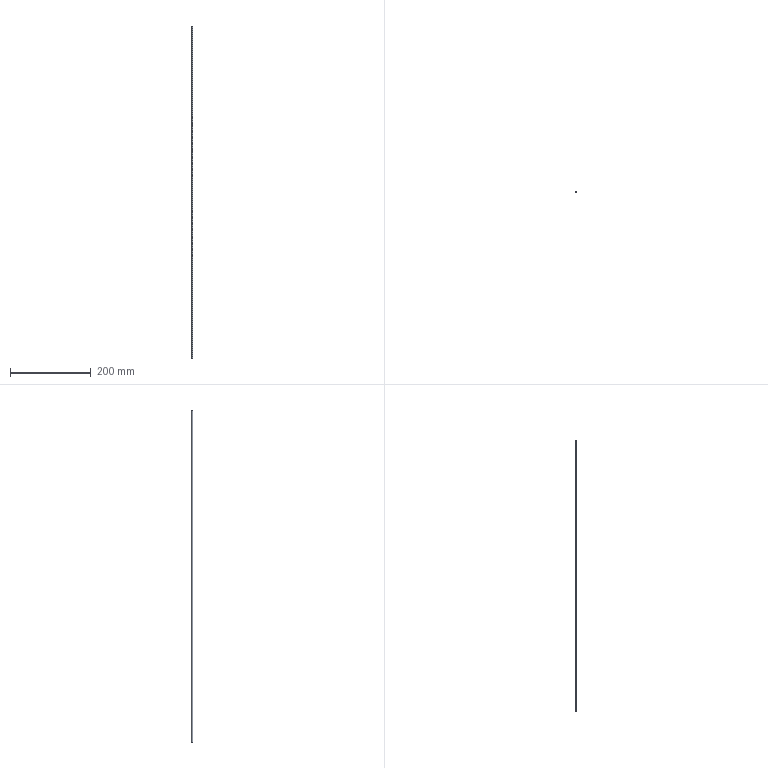Part | STEP file | PZ-G51EP-Part-1 | 1 solid | 4 faces | box 3 x 3 x 823 mm | volume 5817 mm3 | cylinder 2 | plane 2 | commonest cylinder face diameters 3 x2
STEP:
#1=CARTESIAN_POINT('',(0.,5.5,823.));
#2=VERTEX_POINT('',#1);
#3=CARTESIAN_POINT('',(0.,2.5,823.));
#4=VERTEX_POINT('',#3);
#5=CARTESIAN_POINT('',(0.,4.,823.));
#6=DIRECTION('',(0.,0.,-1.));
#7=DIRECTION('',(0.,1.,0.));
#8=AXIS2_PLACEMENT_3D('',#5,#6,#7);
#9=CIRCLE('',#8,1.5);
#10=EDGE_CURVE('',#2,#4,#9,.T.);
#11=ORIENTED_EDGE('',*,*,#10,.T.);
#12=CARTESIAN_POINT('',(0.,2.5,0.));
#13=VERTEX_POINT('',#12);
#14=CARTESIAN_POINT('',(0.,2.5,823.));
#15=DIRECTION('',(0.,0.,-1.));
#16=VECTOR('',#15,1000.);
#17=LINE('',#14,#16);
#18=EDGE_CURVE('',#4,#13,#17,.T.);
#19=ORIENTED_EDGE('',*,*,#18,.T.);
#20=CARTESIAN_POINT('',(0.,5.5,0.));
#21=VERTEX_POINT('',#20);
#22=CARTESIAN_POINT('',(0.,4.,0.));
#23=DIRECTION('',(0.,0.,1.));
#24=DIRECTION('',(0.,-1.,0.));
#25=AXIS2_PLACEMENT_3D('',#22,#23,#24);
#26=CIRCLE('',#25,1.5);
#27=EDGE_CURVE('',#13,#21,#26,.T.);
#28=ORIENTED_EDGE('',*,*,#27,.T.);
#29=CARTESIAN_POINT('',(0.,5.5,823.));
#30=DIRECTION('',(0.,0.,-1.));
#31=VECTOR('',#30,1000.);
#32=LINE('',#29,#31);
#33=EDGE_CURVE('',#2,#21,#32,.T.);
#34=ORIENTED_EDGE('',*,*,#33,.F.);
#35=EDGE_LOOP('',(#11,#19,#28,#34));
#36=FACE_OUTER_BOUND('',#35,.T.);
#37=CARTESIAN_POINT('',(0.,4.,823.));
#38=DIRECTION('',(0.,0.,-1.));
#39=DIRECTION('',(0.,1.,0.));
#40=AXIS2_PLACEMENT_3D('',#37,#38,#39);
#41=CYLINDRICAL_SURFACE('',#40,1.5);
#42=ADVANCED_FACE('',(#36),#41,.T.);
#43=CARTESIAN_POINT('',(0.,4.,0.));
#44=DIRECTION('',(0.,0.,1.));
#45=DIRECTION('',(0.,-1.,0.));
#46=AXIS2_PLACEMENT_3D('',#43,#44,#45);
#47=CIRCLE('',#46,1.5);
#48=EDGE_CURVE('',#21,#13,#47,.T.);
#49=ORIENTED_EDGE('',*,*,#48,.F.);
#50=ORIENTED_EDGE('',*,*,#27,.F.);
#51=EDGE_LOOP('',(#49,#50));
#52=FACE_OUTER_BOUND('',#51,.T.);
#53=CARTESIAN_POINT('',(0.,4.,0.));
#54=DIRECTION('',(0.,0.,-1.));
#55=DIRECTION('',(0.,1.,0.));
#56=AXIS2_PLACEMENT_3D('',#53,#54,#55);
#57=PLANE('',#56);
#58=ADVANCED_FACE('',(#52),#57,.T.);
#59=ORIENTED_EDGE('',*,*,#10,.F.);
#60=CARTESIAN_POINT('',(0.,4.,823.));
#61=DIRECTION('',(0.,0.,-1.));
#62=DIRECTION('',(0.,1.,0.));
#63=AXIS2_PLACEMENT_3D('',#60,#61,#62);
#64=CIRCLE('',#63,1.5);
#65=EDGE_CURVE('',#4,#2,#64,.T.);
#66=ORIENTED_EDGE('',*,*,#65,.F.);
#67=EDGE_LOOP('',(#59,#66));
#68=FACE_OUTER_BOUND('',#67,.T.);
#69=CARTESIAN_POINT('',(0.,4.,823.));
#70=DIRECTION('',(0.,0.,1.));
#71=DIRECTION('',(0.,-1.,0.));
#72=AXIS2_PLACEMENT_3D('',#69,#70,#71);
#73=PLANE('',#72);
#74=ADVANCED_FACE('',(#68),#73,.T.);
#75=ORIENTED_EDGE('',*,*,#18,.F.);
#76=ORIENTED_EDGE('',*,*,#65,.T.);
#77=ORIENTED_EDGE('',*,*,#33,.T.);
#78=ORIENTED_EDGE('',*,*,#48,.T.);
#79=EDGE_LOOP('',(#75,#76,#77,#78));
#80=FACE_OUTER_BOUND('',#79,.T.);
#81=CARTESIAN_POINT('',(0.,4.,823.));
#82=DIRECTION('',(0.,0.,-1.));
#83=DIRECTION('',(0.,1.,0.));
#84=AXIS2_PLACEMENT_3D('',#81,#82,#83);
#85=CYLINDRICAL_SURFACE('',#84,1.5);
#86=ADVANCED_FACE('',(#80),#85,.T.);
#87=CLOSED_SHELL('',(#42,#58,#74,#86));
#88=MANIFOLD_SOLID_BREP('',#87);
#89=CARTESIAN_POINT('',(0.,0.,0.));
#90=DIRECTION('',(0.,0.,1.));
#91=DIRECTION('',(1.,0.,0.));
#92=AXIS2_PLACEMENT_3D('',#89,#90,#91);
#93=(LENGTH_UNIT()NAMED_UNIT(*)SI_UNIT(.MILLI.,.METRE.));
#94=UNCERTAINTY_MEASURE_WITH_UNIT(LENGTH_MEASURE(0.00001),#93,'','');
#95=(NAMED_UNIT(*)PLANE_ANGLE_UNIT()SI_UNIT($,.RADIAN.));
#96=(NAMED_UNIT(*)SI_UNIT($,.STERADIAN.)SOLID_ANGLE_UNIT());
#97=(GEOMETRIC_REPRESENTATION_CONTEXT(3)GLOBAL_UNCERTAINTY_ASSIGNED_CONTEXT((#94))GLOBAL_UNIT_ASSIGNED_CONTEXT((#93,#95,#96))REPRESENTATION_CONTEXT('',''));
#98=ADVANCED_BREP_SHAPE_REPRESENTATION('',(#88,#92),#97);